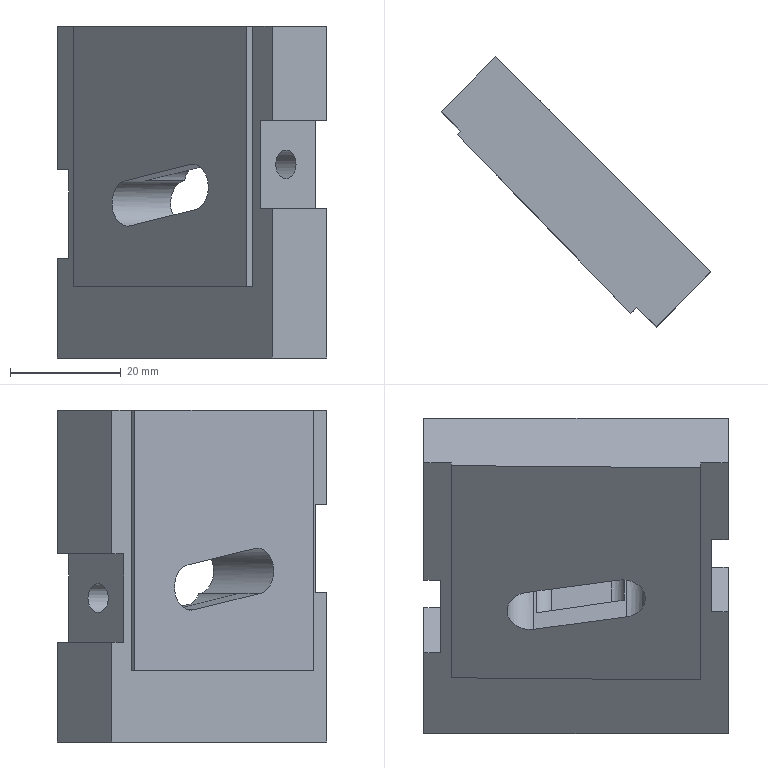Part | STEP file | gslz 2016.10.28-13_id1374_x_t | 1 solid | 38 faces | box 48.79 x 48.79 x 60 mm | volume 42680 mm3 | plane 23 | cylinder 8 | spline 5 | cone 2 | commonest cylinder face diameters 6 x4 5.2 x2 13 x2